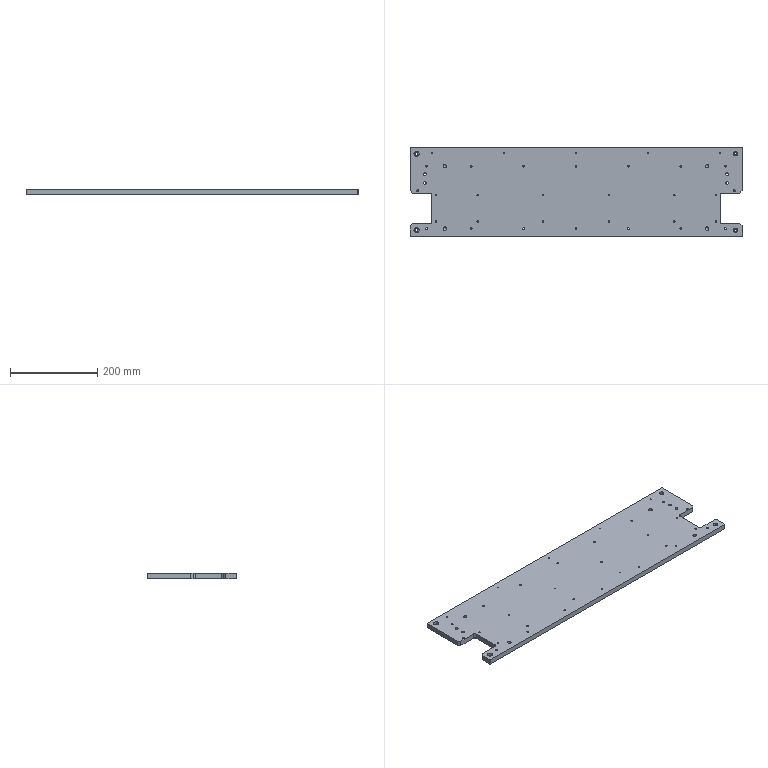Part | SolidWorks | features HoleWzd 8, Chamfer 2, ICE 2, Extrusion 1, Fillet 1 | 1 solid | 166 faces | box 760 x 205 x 12 mm | volume 1773307 mm3 | cylinder 106 | cone 32 | plane 28 | commonest cylinder face diameters 4.2 x28 3.3 x24 6.6 x12 2.5 x10 8 x8 10 x8